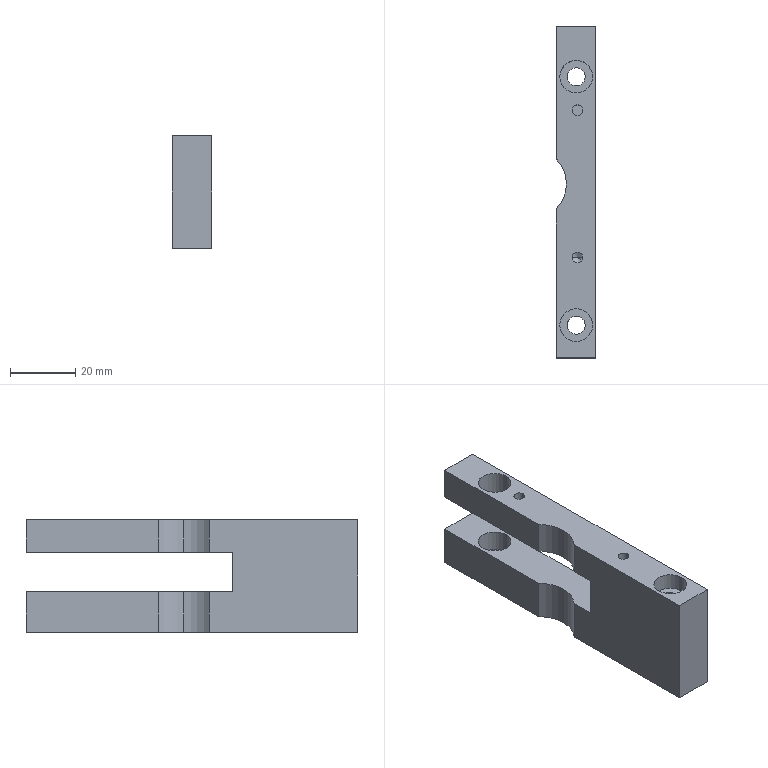Part | STEP file | side block 5 | 1 solid | 34 faces | box 12.1 x 101.5 x 34.5 mm | volume 29782 mm3 | cylinder 18 | plane 14 | cone 2 | commonest cylinder face diameters 10 x6 3.3 x4 5.5 x4 22 x4